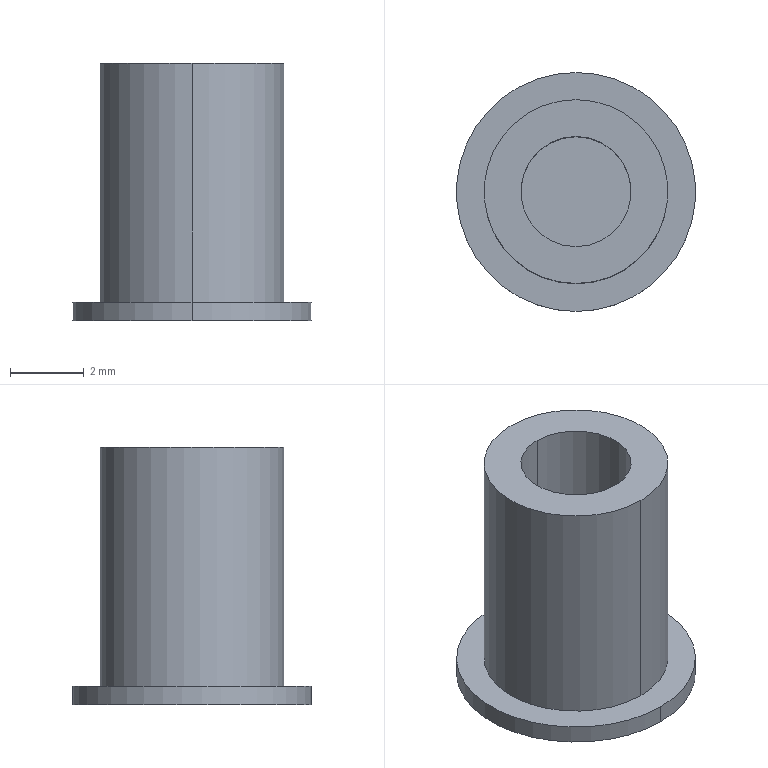Part | STEP file | LRS-150-12_X2_5F00517375-151326 | 1 solid | 10 faces | box 6.5 x 6.5 x 7 mm | volume 95.446 mm3 | cylinder 6 | plane 4 | commonest cylinder face diameters 3 x2 5 x2 6.5 x2
STEP:
#1=CARTESIAN_POINT('',(0.,0.,0.));
#2=DIRECTION('',(0.,0.,1.));
#3=DIRECTION('',(1.,0.,0.));
#4=AXIS2_PLACEMENT_3D('',#1,#2,#3);
#5=CARTESIAN_POINT('',(-289.434,297.675,-6.7));
#6=VERTEX_POINT('',#5);
#7=CARTESIAN_POINT('',(-289.434,294.675,-6.7));
#8=VERTEX_POINT('',#7);
#9=CARTESIAN_POINT('',(-289.434,296.175,-6.7));
#10=DIRECTION('',(0.,0.,1.));
#11=DIRECTION('',(0.,1.,0.));
#12=AXIS2_PLACEMENT_3D('',#9,#10,#11);
#13=CIRCLE('',#12,1.5);
#14=CARTESIAN_POINT('',(-289.434,295.425,-6.7));
#15=DIRECTION('',(0.,0.,-1.));
#16=DIRECTION('',(0.,1.,0.));
#17=AXIS2_PLACEMENT_3D('',#14,#15,#16);
#18=PLANE('',#17);
#19=CARTESIAN_POINT('',(2.25,0.));
#20=CARTESIAN_POINT('',(2.25,-2.598));
#21=CARTESIAN_POINT('',(0.,-1.299));
#22=CARTESIAN_POINT('',(-2.25,0.));
#23=CARTESIAN_POINT('',(0.,1.299));
#24=CARTESIAN_POINT('',(2.25,2.598));
#25=CARTESIAN_POINT('',(2.25,0.));
#26=(BOUNDED_CURVE()B_SPLINE_CURVE(2,(#19,#20,#21,#22,#23,#24,#25),.UNSPECIFIED.,.T.,.F.)B_SPLINE_CURVE_WITH_KNOTS((1,2,2,2,2,1),(-2.094,0.,2.094,4.189,6.283,8.378),.UNSPECIFIED.)CURVE()GEOMETRIC_REPRESENTATION_ITEM()RATIONAL_B_SPLINE_CURVE((1.,0.5,1.,0.5,1.,0.5,1.))REPRESENTATION_ITEM(''));
#27=(GEOMETRIC_REPRESENTATION_CONTEXT(2)PARAMETRIC_REPRESENTATION_CONTEXT()REPRESENTATION_CONTEXT('',''));
#28=DEFINITIONAL_REPRESENTATION('',(#26),#27);
#29=PCURVE('',#18,#28);
#30=CARTESIAN_POINT('',(-289.434,296.175,-1.6));
#31=DIRECTION('',(0.,0.,-1.));
#32=DIRECTION('',(0.,1.,0.));
#33=AXIS2_PLACEMENT_3D('',#30,#31,#32);
#34=CYLINDRICAL_SURFACE('',#33,1.5);
#35=CARTESIAN_POINT('',(6.283,5.1));
#36=DIRECTION('',(-1.,0.));
#37=VECTOR('',#36,1.);
#38=LINE('',#35,#37);
#39=(GEOMETRIC_REPRESENTATION_CONTEXT(2)PARAMETRIC_REPRESENTATION_CONTEXT()REPRESENTATION_CONTEXT('',''));
#40=DEFINITIONAL_REPRESENTATION('',(#38),#39);
#41=PCURVE('',#34,#40);
#42=SURFACE_CURVE('',#13,(#29,#41),.PCURVE_S1.);
#43=EDGE_CURVE('',#6,#8,#42,.T.);
#44=ORIENTED_EDGE('',*,*,#43,.F.);
#45=CARTESIAN_POINT('',(-289.434,296.175,-6.7));
#46=DIRECTION('',(0.,0.,1.));
#47=DIRECTION('',(0.,-1.,0.));
#48=AXIS2_PLACEMENT_3D('',#45,#46,#47);
#49=CIRCLE('',#48,1.5);
#50=CARTESIAN_POINT('',(-0.75,0.));
#51=CARTESIAN_POINT('',(-0.75,2.598));
#52=CARTESIAN_POINT('',(1.5,1.299));
#53=CARTESIAN_POINT('',(3.75,0.));
#54=CARTESIAN_POINT('',(1.5,-1.299));
#55=CARTESIAN_POINT('',(-0.75,-2.598));
#56=CARTESIAN_POINT('',(-0.75,0.));
#57=(BOUNDED_CURVE()B_SPLINE_CURVE(2,(#50,#51,#52,#53,#54,#55,#56),.UNSPECIFIED.,.T.,.F.)B_SPLINE_CURVE_WITH_KNOTS((1,2,2,2,2,1),(-2.094,0.,2.094,4.189,6.283,8.378),.UNSPECIFIED.)CURVE()GEOMETRIC_REPRESENTATION_ITEM()RATIONAL_B_SPLINE_CURVE((1.,0.5,1.,0.5,1.,0.5,1.))REPRESENTATION_ITEM(''));
#58=(GEOMETRIC_REPRESENTATION_CONTEXT(2)PARAMETRIC_REPRESENTATION_CONTEXT()REPRESENTATION_CONTEXT('',''));
#59=DEFINITIONAL_REPRESENTATION('',(#57),#58);
#60=PCURVE('',#18,#59);
#61=CARTESIAN_POINT('',(-289.434,296.175,-1.6));
#62=DIRECTION('',(0.,0.,-1.));
#63=DIRECTION('',(0.,1.,0.));
#64=AXIS2_PLACEMENT_3D('',#61,#62,#63);
#65=CYLINDRICAL_SURFACE('',#64,1.5);
#66=CARTESIAN_POINT('',(3.142,5.1));
#67=DIRECTION('',(-1.,0.));
#68=VECTOR('',#67,1.);
#69=LINE('',#66,#68);
#70=(GEOMETRIC_REPRESENTATION_CONTEXT(2)PARAMETRIC_REPRESENTATION_CONTEXT()REPRESENTATION_CONTEXT('',''));
#71=DEFINITIONAL_REPRESENTATION('',(#69),#70);
#72=PCURVE('',#65,#71);
#73=SURFACE_CURVE('',#49,(#60,#72),.PCURVE_S1.);
#74=EDGE_CURVE('',#8,#6,#73,.T.);
#75=ORIENTED_EDGE('',*,*,#74,.F.);
#76=EDGE_LOOP('',(#44,#75));
#77=FACE_BOUND('',#76,.F.);
#78=ADVANCED_FACE('',(#77),#18,.F.);
#79=ORIENTED_EDGE('',*,*,#43,.T.);
#80=CARTESIAN_POINT('',(-289.434,294.675,0.2));
#81=VERTEX_POINT('',#80);
#82=CARTESIAN_POINT('',(-289.434,294.675,-6.7));
#83=DIRECTION('',(0.,0.,1.));
#84=VECTOR('',#83,1.);
#85=LINE('',#82,#84);
#86=CARTESIAN_POINT('',(3.142,5.1));
#87=DIRECTION('',(0.,-1.));
#88=VECTOR('',#87,1.);
#89=LINE('',#86,#88);
#90=(GEOMETRIC_REPRESENTATION_CONTEXT(2)PARAMETRIC_REPRESENTATION_CONTEXT()REPRESENTATION_CONTEXT('',''));
#91=DEFINITIONAL_REPRESENTATION('',(#89),#90);
#92=PCURVE('',#34,#91);
#93=CARTESIAN_POINT('',(3.142,5.1));
#94=DIRECTION('',(0.,-1.));
#95=VECTOR('',#94,1.);
#96=LINE('',#93,#95);
#97=(GEOMETRIC_REPRESENTATION_CONTEXT(2)PARAMETRIC_REPRESENTATION_CONTEXT()REPRESENTATION_CONTEXT('',''));
#98=DEFINITIONAL_REPRESENTATION('',(#96),#97);
#99=PCURVE('',#65,#98);
#100=SURFACE_CURVE('',#85,(#92,#99),.PCURVE_S1.);
#101=EDGE_CURVE('',#8,#81,#100,.T.);
#102=ORIENTED_EDGE('',*,*,#101,.T.);
#103=CARTESIAN_POINT('',(-289.434,297.675,0.2));
#104=VERTEX_POINT('',#103);
#105=CARTESIAN_POINT('',(-289.434,296.175,0.2));
#106=DIRECTION('',(0.,0.,-1.));
#107=DIRECTION('',(0.,-1.,0.));
#108=AXIS2_PLACEMENT_3D('',#105,#106,#107);
#109=CIRCLE('',#108,1.5);
#110=CARTESIAN_POINT('',(3.142,-1.8));
#111=DIRECTION('',(1.,0.));
#112=VECTOR('',#111,1.);
#113=LINE('',#110,#112);
#114=(GEOMETRIC_REPRESENTATION_CONTEXT(2)PARAMETRIC_REPRESENTATION_CONTEXT()REPRESENTATION_CONTEXT('',''));
#115=DEFINITIONAL_REPRESENTATION('',(#113),#114);
#116=PCURVE('',#34,#115);
#117=CARTESIAN_POINT('',(-289.434,294.175,0.2));
#118=DIRECTION('',(0.,0.,-1.));
#119=DIRECTION('',(0.,1.,0.));
#120=AXIS2_PLACEMENT_3D('',#117,#118,#119);
#121=PLANE('',#120);
#122=CARTESIAN_POINT('',(2.,0.));
#123=DIRECTION('',(-1.,0.));
#124=AXIS2_PLACEMENT_2D('',#122,#123);
#125=CIRCLE('',#124,1.5);
#126=(GEOMETRIC_REPRESENTATION_CONTEXT(2)PARAMETRIC_REPRESENTATION_CONTEXT()REPRESENTATION_CONTEXT('',''));
#127=DEFINITIONAL_REPRESENTATION('',(#125),#126);
#128=PCURVE('',#121,#127);
#129=SURFACE_CURVE('',#109,(#116,#128),.PCURVE_S1.);
#130=EDGE_CURVE('',#81,#104,#129,.T.);
#131=ORIENTED_EDGE('',*,*,#130,.T.);
#132=CARTESIAN_POINT('',(-289.434,297.675,-6.7));
#133=DIRECTION('',(0.,0.,1.));
#134=VECTOR('',#133,1.);
#135=LINE('',#132,#134);
#136=CARTESIAN_POINT('',(6.283,5.1));
#137=DIRECTION('',(0.,-1.));
#138=VECTOR('',#137,1.);
#139=LINE('',#136,#138);
#140=(GEOMETRIC_REPRESENTATION_CONTEXT(2)PARAMETRIC_REPRESENTATION_CONTEXT()REPRESENTATION_CONTEXT('',''));
#141=DEFINITIONAL_REPRESENTATION('',(#139),#140);
#142=PCURVE('',#34,#141);
#143=CARTESIAN_POINT('',(0.,5.1));
#144=DIRECTION('',(0.,-1.));
#145=VECTOR('',#144,1.);
#146=LINE('',#143,#145);
#147=(GEOMETRIC_REPRESENTATION_CONTEXT(2)PARAMETRIC_REPRESENTATION_CONTEXT()REPRESENTATION_CONTEXT('',''));
#148=DEFINITIONAL_REPRESENTATION('',(#146),#147);
#149=PCURVE('',#65,#148);
#150=SURFACE_CURVE('',#135,(#142,#149),.PCURVE_S1.);
#151=EDGE_CURVE('',#6,#104,#150,.T.);
#152=ORIENTED_EDGE('',*,*,#151,.F.);
#153=EDGE_LOOP('',(#79,#102,#131,#152));
#154=FACE_BOUND('',#153,.F.);
#155=ADVANCED_FACE('',(#154),#34,.F.);
#156=CARTESIAN_POINT('',(-289.434,296.175,0.2));
#157=DIRECTION('',(0.,0.,-1.));
#158=DIRECTION('',(0.,1.,0.));
#159=AXIS2_PLACEMENT_3D('',#156,#157,#158);
#160=CIRCLE('',#159,1.5);
#161=CARTESIAN_POINT('',(0.,-1.8));
#162=DIRECTION('',(1.,0.));
#163=VECTOR('',#162,1.);
#164=LINE('',#161,#163);
#165=(GEOMETRIC_REPRESENTATION_CONTEXT(2)PARAMETRIC_REPRESENTATION_CONTEXT()REPRESENTATION_CONTEXT('',''));
#166=DEFINITIONAL_REPRESENTATION('',(#164),#165);
#167=PCURVE('',#65,#166);
#168=CARTESIAN_POINT('',(2.,0.));
#169=DIRECTION('',(1.,0.));
#170=AXIS2_PLACEMENT_2D('',#168,#169);
#171=CIRCLE('',#170,1.5);
#172=(GEOMETRIC_REPRESENTATION_CONTEXT(2)PARAMETRIC_REPRESENTATION_CONTEXT()REPRESENTATION_CONTEXT('',''));
#173=DEFINITIONAL_REPRESENTATION('',(#171),#172);
#174=PCURVE('',#121,#173);
#175=SURFACE_CURVE('',#160,(#167,#174),.PCURVE_S1.);
#176=EDGE_CURVE('',#104,#81,#175,.T.);
#177=ORIENTED_EDGE('',*,*,#176,.T.);
#178=ORIENTED_EDGE('',*,*,#101,.F.);
#179=ORIENTED_EDGE('',*,*,#74,.T.);
#180=ORIENTED_EDGE('',*,*,#151,.T.);
#181=EDGE_LOOP('',(#177,#178,#179,#180));
#182=FACE_BOUND('',#181,.F.);
#183=ADVANCED_FACE('',(#182),#65,.F.);
#184=CARTESIAN_POINT('',(-289.434,298.675,0.2));
#185=VERTEX_POINT('',#184);
#186=CARTESIAN_POINT('',(-289.434,293.675,0.2));
#187=VERTEX_POINT('',#186);
#188=CARTESIAN_POINT('',(-289.434,296.175,0.2));
#189=DIRECTION('',(0.,0.,1.));
#190=DIRECTION('',(0.,1.,0.));
#191=AXIS2_PLACEMENT_3D('',#188,#189,#190);
#192=CIRCLE('',#191,2.5);
#193=CARTESIAN_POINT('',(4.5,0.));
#194=CARTESIAN_POINT('',(4.5,-4.33));
#195=CARTESIAN_POINT('',(0.75,-2.165));
#196=CARTESIAN_POINT('',(-3.,0.));
#197=CARTESIAN_POINT('',(0.75,2.165));
#198=CARTESIAN_POINT('',(4.5,4.33));
#199=CARTESIAN_POINT('',(4.5,0.));
#200=(BOUNDED_CURVE()B_SPLINE_CURVE(2,(#193,#194,#195,#196,#197,#198,#199),.UNSPECIFIED.,.T.,.F.)B_SPLINE_CURVE_WITH_KNOTS((1,2,2,2,2,1),(-2.094,0.,2.094,4.189,6.283,8.378),.UNSPECIFIED.)CURVE()GEOMETRIC_REPRESENTATION_ITEM()RATIONAL_B_SPLINE_CURVE((1.,0.5,1.,0.5,1.,0.5,1.))REPRESENTATION_ITEM(''));
#201=(GEOMETRIC_REPRESENTATION_CONTEXT(2)PARAMETRIC_REPRESENTATION_CONTEXT()REPRESENTATION_CONTEXT('',''));
#202=DEFINITIONAL_REPRESENTATION('',(#200),#201);
#203=PCURVE('',#121,#202);
#204=CARTESIAN_POINT('',(-289.434,296.175,-2.3));
#205=DIRECTION('',(0.,0.,-1.));
#206=DIRECTION('',(0.,1.,0.));
#207=AXIS2_PLACEMENT_3D('',#204,#205,#206);
#208=CYLINDRICAL_SURFACE('',#207,2.5);
#209=CARTESIAN_POINT('',(6.283,-2.5));
#210=DIRECTION('',(-1.,0.));
#211=VECTOR('',#210,1.);
#212=LINE('',#209,#211);
#213=(GEOMETRIC_REPRESENTATION_CONTEXT(2)PARAMETRIC_REPRESENTATION_CONTEXT()REPRESENTATION_CONTEXT('',''));
#214=DEFINITIONAL_REPRESENTATION('',(#212),#213);
#215=PCURVE('',#208,#214);
#216=SURFACE_CURVE('',#192,(#203,#215),.PCURVE_S1.);
#217=EDGE_CURVE('',#185,#187,#216,.T.);
#218=ORIENTED_EDGE('',*,*,#217,.F.);
#219=CARTESIAN_POINT('',(-289.434,296.175,0.2));
#220=DIRECTION('',(0.,0.,1.));
#221=DIRECTION('',(0.,-1.,0.));
#222=AXIS2_PLACEMENT_3D('',#219,#220,#221);
#223=CIRCLE('',#222,2.5);
#224=CARTESIAN_POINT('',(-0.5,0.));
#225=CARTESIAN_POINT('',(-0.5,4.33));
#226=CARTESIAN_POINT('',(3.25,2.165));
#227=CARTESIAN_POINT('',(7.,0.));
#228=CARTESIAN_POINT('',(3.25,-2.165));
#229=CARTESIAN_POINT('',(-0.5,-4.33));
#230=CARTESIAN_POINT('',(-0.5,0.));
#231=(BOUNDED_CURVE()B_SPLINE_CURVE(2,(#224,#225,#226,#227,#228,#229,#230),.UNSPECIFIED.,.T.,.F.)B_SPLINE_CURVE_WITH_KNOTS((1,2,2,2,2,1),(-2.094,0.,2.094,4.189,6.283,8.378),.UNSPECIFIED.)CURVE()GEOMETRIC_REPRESENTATION_ITEM()RATIONAL_B_SPLINE_CURVE((1.,0.5,1.,0.5,1.,0.5,1.))REPRESENTATION_ITEM(''));
#232=(GEOMETRIC_REPRESENTATION_CONTEXT(2)PARAMETRIC_REPRESENTATION_CONTEXT()REPRESENTATION_CONTEXT('',''));
#233=DEFINITIONAL_REPRESENTATION('',(#231),#232);
#234=PCURVE('',#121,#233);
#235=CARTESIAN_POINT('',(-289.434,296.175,-2.3));
#236=DIRECTION('',(0.,0.,-1.));
#237=DIRECTION('',(0.,1.,0.));
#238=AXIS2_PLACEMENT_3D('',#235,#236,#237);
#239=CYLINDRICAL_SURFACE('',#238,2.5);
#240=CARTESIAN_POINT('',(3.142,-2.5));
#241=DIRECTION('',(-1.,0.));
#242=VECTOR('',#241,1.);
#243=LINE('',#240,#242);
#244=(GEOMETRIC_REPRESENTATION_CONTEXT(2)PARAMETRIC_REPRESENTATION_CONTEXT()REPRESENTATION_CONTEXT('',''));
#245=DEFINITIONAL_REPRESENTATION('',(#243),#244);
#246=PCURVE('',#239,#245);
#247=SURFACE_CURVE('',#223,(#234,#246),.PCURVE_S1.);
#248=EDGE_CURVE('',#187,#185,#247,.T.);
#249=ORIENTED_EDGE('',*,*,#248,.F.);
#250=EDGE_LOOP('',(#218,#249));
#251=FACE_BOUND('',#250,.F.);
#252=ORIENTED_EDGE('',*,*,#130,.F.);
#253=ORIENTED_EDGE('',*,*,#176,.F.);
#254=EDGE_LOOP('',(#252,#253));
#255=FACE_BOUND('',#254,.F.);
#256=ADVANCED_FACE('',(#251,#255),#121,.F.);
#257=CARTESIAN_POINT('',(-289.434,298.675,-6.3));
#258=VERTEX_POINT('',#257);
#259=CARTESIAN_POINT('',(-289.434,298.675,0.2));
#260=DIRECTION('',(0.,0.,-1.));
#261=VECTOR('',#260,1.);
#262=LINE('',#259,#261);
#263=CARTESIAN_POINT('',(6.283,-2.5));
#264=DIRECTION('',(0.,1.));
#265=VECTOR('',#264,1.);
#266=LINE('',#263,#265);
#267=(GEOMETRIC_REPRESENTATION_CONTEXT(2)PARAMETRIC_REPRESENTATION_CONTEXT()REPRESENTATION_CONTEXT('',''));
#268=DEFINITIONAL_REPRESENTATION('',(#266),#267);
#269=PCURVE('',#208,#268);
#270=CARTESIAN_POINT('',(0.,-2.5));
#271=DIRECTION('',(0.,1.));
#272=VECTOR('',#271,1.);
#273=LINE('',#270,#272);
#274=(GEOMETRIC_REPRESENTATION_CONTEXT(2)PARAMETRIC_REPRESENTATION_CONTEXT()REPRESENTATION_CONTEXT('',''));
#275=DEFINITIONAL_REPRESENTATION('',(#273),#274);
#276=PCURVE('',#239,#275);
#277=SURFACE_CURVE('',#262,(#269,#276),.PCURVE_S1.);
#278=EDGE_CURVE('',#185,#258,#277,.T.);
#279=ORIENTED_EDGE('',*,*,#278,.T.);
#280=CARTESIAN_POINT('',(-289.434,293.675,-6.3));
#281=VERTEX_POINT('',#280);
#282=CARTESIAN_POINT('',(-289.434,296.175,-6.3));
#283=DIRECTION('',(0.,0.,-1.));
#284=DIRECTION('',(0.,-1.,0.));
#285=AXIS2_PLACEMENT_3D('',#282,#283,#284);
#286=CIRCLE('',#285,2.5);
#287=CARTESIAN_POINT('',(3.142,4.));
#288=DIRECTION('',(1.,0.));
#289=VECTOR('',#288,1.);
#290=LINE('',#287,#289);
#291=(GEOMETRIC_REPRESENTATION_CONTEXT(2)PARAMETRIC_REPRESENTATION_CONTEXT()REPRESENTATION_CONTEXT('',''));
#292=DEFINITIONAL_REPRESENTATION('',(#290),#291);
#293=PCURVE('',#208,#292);
#294=CARTESIAN_POINT('',(-289.434,293.175,-6.3));
#295=DIRECTION('',(0.,0.,-1.));
#296=DIRECTION('',(0.,1.,0.));
#297=AXIS2_PLACEMENT_3D('',#294,#295,#296);
#298=PLANE('',#297);
#299=CARTESIAN_POINT('',(3.,0.));
#300=DIRECTION('',(-1.,0.));
#301=AXIS2_PLACEMENT_2D('',#299,#300);
#302=CIRCLE('',#301,2.5);
#303=(GEOMETRIC_REPRESENTATION_CONTEXT(2)PARAMETRIC_REPRESENTATION_CONTEXT()REPRESENTATION_CONTEXT('',''));
#304=DEFINITIONAL_REPRESENTATION('',(#302),#303);
#305=PCURVE('',#298,#304);
#306=SURFACE_CURVE('',#286,(#293,#305),.PCURVE_S1.);
#307=EDGE_CURVE('',#281,#258,#306,.T.);
#308=ORIENTED_EDGE('',*,*,#307,.F.);
#309=CARTESIAN_POINT('',(-289.434,293.675,0.2));
#310=DIRECTION('',(0.,0.,-1.));
#311=VECTOR('',#310,1.);
#312=LINE('',#309,#311);
#313=CARTESIAN_POINT('',(3.142,-2.5));
#314=DIRECTION('',(0.,1.));
#315=VECTOR('',#314,1.);
#316=LINE('',#313,#315);
#317=(GEOMETRIC_REPRESENTATION_CONTEXT(2)PARAMETRIC_REPRESENTATION_CONTEXT()REPRESENTATION_CONTEXT('',''));
#318=DEFINITIONAL_REPRESENTATION('',(#316),#317);
#319=PCURVE('',#208,#318);
#320=CARTESIAN_POINT('',(3.142,-2.5));
#321=DIRECTION('',(0.,1.));
#322=VECTOR('',#321,1.);
#323=LINE('',#320,#322);
#324=(GEOMETRIC_REPRESENTATION_CONTEXT(2)PARAMETRIC_REPRESENTATION_CONTEXT()REPRESENTATION_CONTEXT('',''));
#325=DEFINITIONAL_REPRESENTATION('',(#323),#324);
#326=PCURVE('',#239,#325);
#327=SURFACE_CURVE('',#312,(#319,#326),.PCURVE_S1.);
#328=EDGE_CURVE('',#187,#281,#327,.T.);
#329=ORIENTED_EDGE('',*,*,#328,.F.);
#330=ORIENTED_EDGE('',*,*,#217,.F.);
#331=EDGE_LOOP('',(#279,#308,#329,#330));
#332=FACE_BOUND('',#331,.T.);
#333=ADVANCED_FACE('',(#332),#208,.T.);
#334=CARTESIAN_POINT('',(-289.434,296.175,-6.3));
#335=DIRECTION('',(0.,0.,-1.));
#336=DIRECTION('',(0.,1.,0.));
#337=AXIS2_PLACEMENT_3D('',#334,#335,#336);
#338=CIRCLE('',#337,2.5);
#339=CARTESIAN_POINT('',(0.,4.));
#340=DIRECTION('',(1.,0.));
#341=VECTOR('',#340,1.);
#342=LINE('',#339,#341);
#343=(GEOMETRIC_REPRESENTATION_CONTEXT(2)PARAMETRIC_REPRESENTATION_CONTEXT()REPRESENTATION_CONTEXT('',''));
#344=DEFINITIONAL_REPRESENTATION('',(#342),#343);
#345=PCURVE('',#239,#344);
#346=CARTESIAN_POINT('',(3.,0.));
#347=DIRECTION('',(1.,0.));
#348=AXIS2_PLACEMENT_2D('',#346,#347);
#349=CIRCLE('',#348,2.5);
#350=(GEOMETRIC_REPRESENTATION_CONTEXT(2)PARAMETRIC_REPRESENTATION_CONTEXT()REPRESENTATION_CONTEXT('',''));
#351=DEFINITIONAL_REPRESENTATION('',(#349),#350);
#352=PCURVE('',#298,#351);
#353=SURFACE_CURVE('',#338,(#345,#352),.PCURVE_S1.);
#354=EDGE_CURVE('',#258,#281,#353,.T.);
#355=ORIENTED_EDGE('',*,*,#354,.F.);
#356=ORIENTED_EDGE('',*,*,#278,.F.);
#357=ORIENTED_EDGE('',*,*,#248,.F.);
#358=ORIENTED_EDGE('',*,*,#328,.T.);
#359=EDGE_LOOP('',(#355,#356,#357,#358));
#360=FACE_BOUND('',#359,.T.);
#361=ADVANCED_FACE('',(#360),#239,.T.);
#362=CARTESIAN_POINT('',(-289.434,299.425,-6.3));
#363=VERTEX_POINT('',#362);
#364=CARTESIAN_POINT('',(-289.434,292.925,-6.3));
#365=VERTEX_POINT('',#364);
#366=CARTESIAN_POINT('',(-289.434,296.175,-6.3));
#367=DIRECTION('',(0.,0.,1.));
#368=DIRECTION('',(0.,1.,0.));
#369=AXIS2_PLACEMENT_3D('',#366,#367,#368);
#370=CIRCLE('',#369,3.25);
#371=CARTESIAN_POINT('',(6.25,0.));
#372=CARTESIAN_POINT('',(6.25,-5.629));
#373=CARTESIAN_POINT('',(1.375,-2.815));
#374=CARTESIAN_POINT('',(-3.5,0.));
#375=CARTESIAN_POINT('',(1.375,2.815));
#376=CARTESIAN_POINT('',(6.25,5.629));
#377=CARTESIAN_POINT('',(6.25,0.));
#378=(BOUNDED_CURVE()B_SPLINE_CURVE(2,(#371,#372,#373,#374,#375,#376,#377),.UNSPECIFIED.,.T.,.F.)B_SPLINE_CURVE_WITH_KNOTS((1,2,2,2,2,1),(-2.094,0.,2.094,4.189,6.283,8.378),.UNSPECIFIED.)CURVE()GEOMETRIC_REPRESENTATION_ITEM()RATIONAL_B_SPLINE_CURVE((1.,0.5,1.,0.5,1.,0.5,1.))REPRESENTATION_ITEM(''));
#379=(GEOMETRIC_REPRESENTATION_CONTEXT(2)PARAMETRIC_REPRESENTATION_CONTEXT()REPRESENTATION_CONTEXT('',''));
#380=DEFINITIONAL_REPRESENTATION('',(#378),#379);
#381=PCURVE('',#298,#380);
#382=CARTESIAN_POINT('',(-289.434,296.175,-7.3));
#383=DIRECTION('',(0.,0.,-1.));
#384=DIRECTION('',(0.,1.,0.));
#385=AXIS2_PLACEMENT_3D('',#382,#383,#384);
#386=CYLINDRICAL_SURFACE('',#385,3.25);
#387=CARTESIAN_POINT('',(6.283,-1.));
#388=DIRECTION('',(-1.,0.));
#389=VECTOR('',#388,1.);
#390=LINE('',#387,#389);
#391=(GEOMETRIC_REPRESENTATION_CONTEXT(2)PARAMETRIC_REPRESENTATION_CONTEXT()REPRESENTATION_CONTEXT('',''));
#392=DEFINITIONAL_REPRESENTATION('',(#390),#391);
#393=PCURVE('',#386,#392);
#394=SURFACE_CURVE('',#370,(#381,#393),.PCURVE_S1.);
#395=EDGE_CURVE('',#363,#365,#394,.T.);
#396=ORIENTED_EDGE('',*,*,#395,.F.);
#397=CARTESIAN_POINT('',(-289.434,296.175,-6.3));
#398=DIRECTION('',(0.,0.,1.));
#399=DIRECTION('',(0.,-1.,0.));
#400=AXIS2_PLACEMENT_3D('',#397,#398,#399);
#401=CIRCLE('',#400,3.25);
#402=CARTESIAN_POINT('',(-0.25,0.));
#403=CARTESIAN_POINT('',(-0.25,5.629));
#404=CARTESIAN_POINT('',(4.625,2.815));
#405=CARTESIAN_POINT('',(9.5,0.));
#406=CARTESIAN_POINT('',(4.625,-2.815));
#407=CARTESIAN_POINT('',(-0.25,-5.629));
#408=CARTESIAN_POINT('',(-0.25,0.));
#409=(BOUNDED_CURVE()B_SPLINE_CURVE(2,(#402,#403,#404,#405,#406,#407,#408),.UNSPECIFIED.,.T.,.F.)B_SPLINE_CURVE_WITH_KNOTS((1,2,2,2,2,1),(-2.094,0.,2.094,4.189,6.283,8.378),.UNSPECIFIED.)CURVE()GEOMETRIC_REPRESENTATION_ITEM()RATIONAL_B_SPLINE_CURVE((1.,0.5,1.,0.5,1.,0.5,1.))REPRESENTATION_ITEM(''));
#410=(GEOMETRIC_REPRESENTATION_CONTEXT(2)PARAMETRIC_REPRESENTATION_CONTEXT()REPRESENTATION_CONTEXT('',''));
#411=DEFINITIONAL_REPRESENTATION('',(#409),#410);
#412=PCURVE('',#298,#411);
#413=CARTESIAN_POINT('',(-289.434,296.175,-7.3));
#414=DIRECTION('',(0.,0.,-1.));
#415=DIRECTION('',(0.,1.,0.));
#416=AXIS2_PLACEMENT_3D('',#413,#414,#415);
#417=CYLINDRICAL_SURFACE('',#416,3.25);
#418=CARTESIAN_POINT('',(3.142,-1.));
#419=DIRECTION('',(-1.,0.));
#420=VECTOR('',#419,1.);
#421=LINE('',#418,#420);
#422=(GEOMETRIC_REPRESENTATION_CONTEXT(2)PARAMETRIC_REPRESENTATION_CONTEXT()REPRESENTATION_CONTEXT('',''));
#423=DEFINITIONAL_REPRESENTATION('',(#421),#422);
#424=PCURVE('',#417,#423);
#425=SURFACE_CURVE('',#401,(#412,#424),.PCURVE_S1.);
#426=EDGE_CURVE('',#365,#363,#425,.T.);
#427=ORIENTED_EDGE('',*,*,#426,.F.);
#428=EDGE_LOOP('',(#396,#427));
#429=FACE_BOUND('',#428,.F.);
#430=ORIENTED_EDGE('',*,*,#307,.F.);
#431=ORIENTED_EDGE('',*,*,#354,.F.);
#432=EDGE_LOOP('',(#430,#431));
#433=FACE_BOUND('',#432,.F.);
#434=ADVANCED_FACE('',(#429,#433),#298,.F.);
#435=CARTESIAN_POINT('',(-289.434,299.425,-6.8));
#436=VERTEX_POINT('',#435);
#437=CARTESIAN_POINT('',(-289.434,299.425,-6.3));
#438=DIRECTION('',(0.,0.,-1.));
#439=VECTOR('',#438,1.);
#440=LINE('',#437,#439);
#441=CARTESIAN_POINT('',(6.283,-1.));
#442=DIRECTION('',(0.,1.));
#443=VECTOR('',#442,1.);
#444=LINE('',#441,#443);
#445=(GEOMETRIC_REPRESENTATION_CONTEXT(2)PARAMETRIC_REPRESENTATION_CONTEXT()REPRESENTATION_CONTEXT('',''));
#446=DEFINITIONAL_REPRESENTATION('',(#444),#445);
#447=PCURVE('',#386,#446);
#448=CARTESIAN_POINT('',(0.,-1.));
#449=DIRECTION('',(0.,1.));
#450=VECTOR('',#449,1.);
#451=LINE('',#448,#450);
#452=(GEOMETRIC_REPRESENTATION_CONTEXT(2)PARAMETRIC_REPRESENTATION_CONTEXT()REPRESENTATION_CONTEXT('',''));
#453=DEFINITIONAL_REPRESENTATION('',(#451),#452);
#454=PCURVE('',#417,#453);
#455=SURFACE_CURVE('',#440,(#447,#454),.PCURVE_S1.);
#456=EDGE_CURVE('',#363,#436,#455,.T.);
#457=ORIENTED_EDGE('',*,*,#456,.T.);
#458=CARTESIAN_POINT('',(-289.434,292.925,-6.8));
#459=VERTEX_POINT('',#458);
#460=CARTESIAN_POINT('',(-289.434,296.175,-6.8));
#461=DIRECTION('',(0.,0.,-1.));
#462=DIRECTION('',(0.,-1.,0.));
#463=AXIS2_PLACEMENT_3D('',#460,#461,#462);
#464=CIRCLE('',#463,3.25);
#465=CARTESIAN_POINT('',(3.142,-0.5));
#466=DIRECTION('',(1.,0.));
#467=VECTOR('',#466,1.);
#468=LINE('',#465,#467);
#469=(GEOMETRIC_REPRESENTATION_CONTEXT(2)PARAMETRIC_REPRESENTATION_CONTEXT()REPRESENTATION_CONTEXT('',''));
#470=DEFINITIONAL_REPRESENTATION('',(#468),#469);
#471=PCURVE('',#386,#470);
#472=CARTESIAN_POINT('',(-520.434,303.645,-6.8));
#473=DIRECTION('',(0.,0.,-1.));
#474=DIRECTION('',(0.,-1.,0.));
#475=AXIS2_PLACEMENT_3D('',#472,#473,#474);
#476=PLANE('',#475);
#477=CARTESIAN_POINT('',(7.47,-231.));
#478=DIRECTION('',(1.,0.));
#479=AXIS2_PLACEMENT_2D('',#477,#478);
#480=CIRCLE('',#479,3.25);
#481=(GEOMETRIC_REPRESENTATION_CONTEXT(2)PARAMETRIC_REPRESENTATION_CONTEXT()REPRESENTATION_CONTEXT('',''));
#482=DEFINITIONAL_REPRESENTATION('',(#480),#481);
#483=PCURVE('',#476,#482);
#484=SURFACE_CURVE('',#464,(#471,#483),.PCURVE_S1.);
#485=EDGE_CURVE('',#459,#436,#484,.T.);
#486=ORIENTED_EDGE('',*,*,#485,.F.);
#487=CARTESIAN_POINT('',(-289.434,292.925,-6.3));
#488=DIRECTION('',(0.,0.,-1.));
#489=VECTOR('',#488,1.);
#490=LINE('',#487,#489);
#491=CARTESIAN_POINT('',(3.142,-1.));
#492=DIRECTION('',(0.,1.));
#493=VECTOR('',#492,1.);
#494=LINE('',#491,#493);
#495=(GEOMETRIC_REPRESENTATION_CONTEXT(2)PARAMETRIC_REPRESENTATION_CONTEXT()REPRESENTATION_CONTEXT('',''));
#496=DEFINITIONAL_REPRESENTATION('',(#494),#495);
#497=PCURVE('',#386,#496);
#498=CARTESIAN_POINT('',(3.142,-1.));
#499=DIRECTION('',(0.,1.));
#500=VECTOR('',#499,1.);
#501=LINE('',#498,#500);
#502=(GEOMETRIC_REPRESENTATION_CONTEXT(2)PARAMETRIC_REPRESENTATION_CONTEXT()REPRESENTATION_CONTEXT('',''));
#503=DEFINITIONAL_REPRESENTATION('',(#501),#502);
#504=PCURVE('',#417,#503);
#505=SURFACE_CURVE('',#490,(#497,#504),.PCURVE_S1.);
#506=EDGE_CURVE('',#365,#459,#505,.T.);
#507=ORIENTED_EDGE('',*,*,#506,.F.);
#508=ORIENTED_EDGE('',*,*,#395,.F.);
#509=EDGE_LOOP('',(#457,#486,#507,#508));
#510=FACE_BOUND('',#509,.T.);
#511=ADVANCED_FACE('',(#510),#386,.T.);
#512=CARTESIAN_POINT('',(-289.434,296.175,-6.8));
#513=DIRECTION('',(0.,0.,-1.));
#514=DIRECTION('',(0.,1.,0.));
#515=AXIS2_PLACEMENT_3D('',#512,#513,#514);
#516=CIRCLE('',#515,3.25);
#517=CARTESIAN_POINT('',(0.,-0.5));
#518=DIRECTION('',(1.,0.));
#519=VECTOR('',#518,1.);
#520=LINE('',#517,#519);
#521=(GEOMETRIC_REPRESENTATION_CONTEXT(2)PARAMETRIC_REPRESENTATION_CONTEXT()REPRESENTATION_CONTEXT('',''));
#522=DEFINITIONAL_REPRESENTATION('',(#520),#521);
#523=PCURVE('',#417,#522);
#524=CARTESIAN_POINT('',(7.47,-231.));
#525=DIRECTION('',(-1.,0.));
#526=AXIS2_PLACEMENT_2D('',#524,#525);
#527=CIRCLE('',#526,3.25);
#528=(GEOMETRIC_REPRESENTATION_CONTEXT(2)PARAMETRIC_REPRESENTATION_CONTEXT()REPRESENTATION_CONTEXT('',''));
#529=DEFINITIONAL_REPRESENTATION('',(#527),#528);
#530=PCURVE('',#476,#529);
#531=SURFACE_CURVE('',#516,(#523,#530),.PCURVE_S1.);
#532=EDGE_CURVE('',#436,#459,#531,.T.);
#533=ORIENTED_EDGE('',*,*,#532,.F.);
#534=ORIENTED_EDGE('',*,*,#456,.F.);
#535=ORIENTED_EDGE('',*,*,#426,.F.);
#536=ORIENTED_EDGE('',*,*,#506,.T.);
#537=EDGE_LOOP('',(#533,#534,#535,#536));
#538=FACE_BOUND('',#537,.T.);
#539=ADVANCED_FACE('',(#538),#417,.T.);
#540=ORIENTED_EDGE('',*,*,#485,.F.);
#541=ORIENTED_EDGE('',*,*,#532,.F.);
#542=EDGE_LOOP('',(#540,#541));
#543=FACE_BOUND('',#542,.F.);
#544=ADVANCED_FACE('',(#543),#476,.T.);
#545=CLOSED_SHELL('',(#78,#155,#183,#256,#333,#361,#434,#511,#539,#544));
#546=MANIFOLD_SOLID_BREP('',#545);
#547=(LENGTH_UNIT()NAMED_UNIT(*)SI_UNIT(.MILLI.,.METRE.));
#548=UNCERTAINTY_MEASURE_WITH_UNIT(LENGTH_MEASURE(0.0000001),#547,'','');
#549=(NAMED_UNIT(*)PLANE_ANGLE_UNIT()SI_UNIT($,.RADIAN.));
#550=(NAMED_UNIT(*)SI_UNIT($,.STERADIAN.)SOLID_ANGLE_UNIT());
#551=(GEOMETRIC_REPRESENTATION_CONTEXT(3)GLOBAL_UNCERTAINTY_ASSIGNED_CONTEXT((#548))GLOBAL_UNIT_ASSIGNED_CONTEXT((#547,#549,#550))REPRESENTATION_CONTEXT('',''));
#552=ADVANCED_BREP_SHAPE_REPRESENTATION('',(#4,#546),#551);